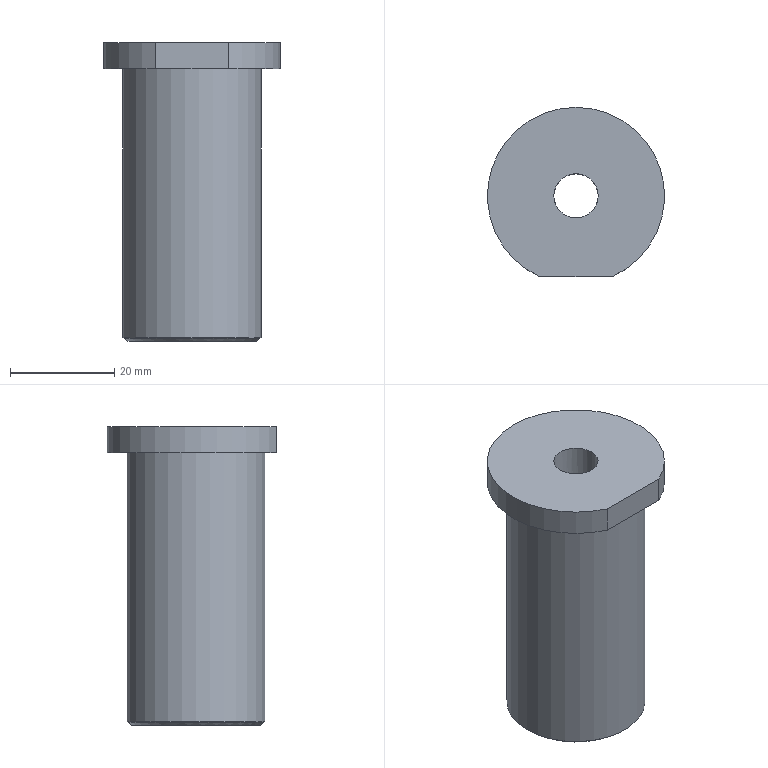Part | STEP file | SLIDE2-INSERT2_id610_x_t | 1 solid | 36 faces | box 34 x 32.5 x 57.321 mm | volume 25904 mm3 | plane 30 | cylinder 3 | other 2 | cone 1 | commonest cylinder face diameters 8.5 x1 26.5 x1 34 x1
STEP:
#1=CARTESIAN_POINT('',(18.501,-6.,56.682));
#2=VERTEX_POINT('',#1);
#3=CARTESIAN_POINT('',(18.617,-6.,56.682));
#4=VERTEX_POINT('',#3);
#5=CARTESIAN_POINT('',(22.656,-6.,56.682));
#6=DIRECTION('',(1.,0.,0.));
#7=VECTOR('',#6,1.);
#8=LINE('',#5,#7);
#9=EDGE_CURVE('',#2,#4,#8,.T.);
#10=ORIENTED_EDGE('',*,*,#9,.F.);
#11=CARTESIAN_POINT('',(18.501,-4.25,56.682));
#12=VERTEX_POINT('',#11);
#13=CARTESIAN_POINT('',(18.501,-6.,56.682));
#14=DIRECTION('',(0.,-1.,0.));
#15=VECTOR('',#14,1.);
#16=LINE('',#13,#15);
#17=EDGE_CURVE('',#12,#2,#16,.T.);
#18=ORIENTED_EDGE('',*,*,#17,.F.);
#19=CARTESIAN_POINT('',(18.617,-4.25,56.682));
#20=VERTEX_POINT('',#19);
#21=CARTESIAN_POINT('',(18.559,0.,56.682));
#22=DIRECTION('',(0.,0.,-1.));
#23=DIRECTION('',(1.,0.,0.));
#24=AXIS2_PLACEMENT_3D('',#21,#22,#23);
#25=CIRCLE('',#24,4.25);
#26=EDGE_CURVE('',#20,#12,#25,.T.);
#27=ORIENTED_EDGE('',*,*,#26,.F.);
#28=CARTESIAN_POINT('',(18.617,-6.,56.682));
#29=DIRECTION('',(0.,1.,0.));
#30=VECTOR('',#29,1.);
#31=LINE('',#28,#30);
#32=EDGE_CURVE('',#4,#20,#31,.T.);
#33=ORIENTED_EDGE('',*,*,#32,.F.);
#34=EDGE_LOOP('',(#10,#18,#27,#33));
#35=FACE_OUTER_BOUND('',#34,.T.);
#36=CARTESIAN_POINT('',(22.656,-6.,56.682));
#37=DIRECTION('',(0.,0.,1.));
#38=DIRECTION('',(1.,0.,0.));
#39=AXIS2_PLACEMENT_3D('',#36,#37,#38);
#40=PLANE('',#39);
#41=ADVANCED_FACE('',(#35),#40,.F.);
#42=CARTESIAN_POINT('',(18.501,6.,56.682));
#43=VERTEX_POINT('',#42);
#44=CARTESIAN_POINT('',(18.501,4.25,56.682));
#45=VERTEX_POINT('',#44);
#46=CARTESIAN_POINT('',(18.501,6.,56.682));
#47=DIRECTION('',(0.,-1.,0.));
#48=VECTOR('',#47,1.);
#49=LINE('',#46,#48);
#50=EDGE_CURVE('',#43,#45,#49,.T.);
#51=ORIENTED_EDGE('',*,*,#50,.F.);
#52=CARTESIAN_POINT('',(18.617,6.,56.682));
#53=VERTEX_POINT('',#52);
#54=CARTESIAN_POINT('',(22.656,6.,56.682));
#55=DIRECTION('',(-1.,0.,0.));
#56=VECTOR('',#55,1.);
#57=LINE('',#54,#56);
#58=EDGE_CURVE('',#53,#43,#57,.T.);
#59=ORIENTED_EDGE('',*,*,#58,.F.);
#60=CARTESIAN_POINT('',(18.617,4.25,56.682));
#61=VERTEX_POINT('',#60);
#62=CARTESIAN_POINT('',(18.617,6.,56.682));
#63=DIRECTION('',(0.,1.,0.));
#64=VECTOR('',#63,1.);
#65=LINE('',#62,#64);
#66=EDGE_CURVE('',#61,#53,#65,.T.);
#67=ORIENTED_EDGE('',*,*,#66,.F.);
#68=CARTESIAN_POINT('',(18.559,0.,56.682));
#69=DIRECTION('',(0.,0.,-1.));
#70=DIRECTION('',(1.,0.,0.));
#71=AXIS2_PLACEMENT_3D('',#68,#69,#70);
#72=CIRCLE('',#71,4.25);
#73=EDGE_CURVE('',#45,#61,#72,.T.);
#74=ORIENTED_EDGE('',*,*,#73,.F.);
#75=EDGE_LOOP('',(#51,#59,#67,#74));
#76=FACE_OUTER_BOUND('',#75,.T.);
#77=CARTESIAN_POINT('',(22.656,-6.,56.682));
#78=DIRECTION('',(0.,0.,1.));
#79=DIRECTION('',(1.,0.,0.));
#80=AXIS2_PLACEMENT_3D('',#77,#78,#79);
#81=PLANE('',#80);
#82=ADVANCED_FACE('',(#76),#81,.F.);
#83=CARTESIAN_POINT('',(25.977,-6.,18.682));
#84=VERTEX_POINT('',#83);
#85=CARTESIAN_POINT('',(25.977,-4.1,18.682));
#86=VERTEX_POINT('',#85);
#87=CARTESIAN_POINT('',(25.977,-6.,18.682));
#88=DIRECTION('',(0.,1.,0.));
#89=VECTOR('',#88,1.);
#90=LINE('',#87,#89);
#91=EDGE_CURVE('',#84,#86,#90,.T.);
#92=ORIENTED_EDGE('',*,*,#91,.F.);
#93=CARTESIAN_POINT('',(23.957,-6.,18.682));
#94=VERTEX_POINT('',#93);
#95=CARTESIAN_POINT('',(-30.,-6.,18.682));
#96=DIRECTION('',(-1.,0.,0.));
#97=VECTOR('',#96,1.);
#98=LINE('',#95,#97);
#99=EDGE_CURVE('',#84,#94,#98,.T.);
#100=ORIENTED_EDGE('',*,*,#99,.T.);
#101=CARTESIAN_POINT('',(23.957,-4.1,18.682));
#102=VERTEX_POINT('',#101);
#103=CARTESIAN_POINT('',(23.957,-6.,18.682));
#104=DIRECTION('',(0.,-1.,0.));
#105=VECTOR('',#104,1.);
#106=LINE('',#103,#105);
#107=EDGE_CURVE('',#102,#94,#106,.T.);
#108=ORIENTED_EDGE('',*,*,#107,.F.);
#109=CARTESIAN_POINT('',(-30.,-4.1,18.682));
#110=DIRECTION('',(-1.,0.,0.));
#111=VECTOR('',#110,1.);
#112=LINE('',#109,#111);
#113=EDGE_CURVE('',#86,#102,#112,.T.);
#114=ORIENTED_EDGE('',*,*,#113,.F.);
#115=EDGE_LOOP('',(#92,#100,#108,#114));
#116=FACE_OUTER_BOUND('',#115,.T.);
#117=CARTESIAN_POINT('',(25.977,-6.,18.682));
#118=DIRECTION('',(0.,0.,-1.));
#119=DIRECTION('',(-1.,0.,0.));
#120=AXIS2_PLACEMENT_3D('',#117,#118,#119);
#121=PLANE('',#120);
#122=ADVANCED_FACE('',(#116),#121,.T.);
#123=CARTESIAN_POINT('',(13.16,-6.,18.682));
#124=VERTEX_POINT('',#123);
#125=CARTESIAN_POINT('',(13.16,-4.1,18.682));
#126=VERTEX_POINT('',#125);
#127=CARTESIAN_POINT('',(13.16,-6.,18.682));
#128=DIRECTION('',(0.,1.,0.));
#129=VECTOR('',#128,1.);
#130=LINE('',#127,#129);
#131=EDGE_CURVE('',#124,#126,#130,.T.);
#132=ORIENTED_EDGE('',*,*,#131,.F.);
#133=CARTESIAN_POINT('',(11.14,-6.,18.682));
#134=VERTEX_POINT('',#133);
#135=CARTESIAN_POINT('',(-30.,-6.,18.682));
#136=DIRECTION('',(-1.,0.,0.));
#137=VECTOR('',#136,1.);
#138=LINE('',#135,#137);
#139=EDGE_CURVE('',#124,#134,#138,.T.);
#140=ORIENTED_EDGE('',*,*,#139,.T.);
#141=CARTESIAN_POINT('',(11.14,-4.1,18.682));
#142=VERTEX_POINT('',#141);
#143=CARTESIAN_POINT('',(11.14,-6.,18.682));
#144=DIRECTION('',(0.,-1.,0.));
#145=VECTOR('',#144,1.);
#146=LINE('',#143,#145);
#147=EDGE_CURVE('',#142,#134,#146,.T.);
#148=ORIENTED_EDGE('',*,*,#147,.F.);
#149=CARTESIAN_POINT('',(-30.,-4.1,18.682));
#150=DIRECTION('',(-1.,0.,0.));
#151=VECTOR('',#150,1.);
#152=LINE('',#149,#151);
#153=EDGE_CURVE('',#126,#142,#152,.T.);
#154=ORIENTED_EDGE('',*,*,#153,.F.);
#155=EDGE_LOOP('',(#132,#140,#148,#154));
#156=FACE_OUTER_BOUND('',#155,.T.);
#157=CARTESIAN_POINT('',(13.16,-6.,18.682));
#158=DIRECTION('',(0.,0.,-1.));
#159=DIRECTION('',(-1.,0.,0.));
#160=AXIS2_PLACEMENT_3D('',#157,#158,#159);
#161=PLANE('',#160);
#162=ADVANCED_FACE('',(#156),#161,.T.);
#163=ORIENTED_EDGE('',*,*,#147,.T.);
#164=CARTESIAN_POINT('',(16.481,-6.,56.682));
#165=VERTEX_POINT('',#164);
#166=CARTESIAN_POINT('',(11.14,-6.,18.682));
#167=DIRECTION('',(0.1392,0.,0.9903));
#168=VECTOR('',#167,1.);
#169=LINE('',#166,#168);
#170=EDGE_CURVE('',#134,#165,#169,.T.);
#171=ORIENTED_EDGE('',*,*,#170,.T.);
#172=CARTESIAN_POINT('',(16.481,-4.1,56.682));
#173=VERTEX_POINT('',#172);
#174=CARTESIAN_POINT('',(16.481,-6.,56.682));
#175=DIRECTION('',(0.,1.,0.));
#176=VECTOR('',#175,1.);
#177=LINE('',#174,#176);
#178=EDGE_CURVE('',#165,#173,#177,.T.);
#179=ORIENTED_EDGE('',*,*,#178,.T.);
#180=CARTESIAN_POINT('',(11.14,-4.1,18.682));
#181=DIRECTION('',(0.1392,0.,0.9903));
#182=VECTOR('',#181,1.);
#183=LINE('',#180,#182);
#184=EDGE_CURVE('',#142,#173,#183,.T.);
#185=ORIENTED_EDGE('',*,*,#184,.F.);
#186=EDGE_LOOP('',(#163,#171,#179,#185));
#187=FACE_OUTER_BOUND('',#186,.T.);
#188=CARTESIAN_POINT('',(11.14,-6.,18.682));
#189=DIRECTION('',(-0.9903,0.,0.1392));
#190=DIRECTION('',(0.1392,0.,0.9903));
#191=AXIS2_PLACEMENT_3D('',#188,#189,#190);
#192=PLANE('',#191);
#193=ADVANCED_FACE('',(#187),#192,.T.);
#194=CARTESIAN_POINT('',(20.636,-4.1,56.682));
#195=VERTEX_POINT('',#194);
#196=CARTESIAN_POINT('',(20.636,-6.,56.682));
#197=VERTEX_POINT('',#196);
#198=CARTESIAN_POINT('',(20.636,-6.,56.682));
#199=DIRECTION('',(0.,-1.,0.));
#200=VECTOR('',#199,1.);
#201=LINE('',#198,#200);
#202=EDGE_CURVE('',#195,#197,#201,.T.);
#203=ORIENTED_EDGE('',*,*,#202,.T.);
#204=CARTESIAN_POINT('',(20.636,-6.,56.682));
#205=DIRECTION('',(0.1392,0.,-0.9903));
#206=VECTOR('',#205,1.);
#207=LINE('',#204,#206);
#208=EDGE_CURVE('',#197,#84,#207,.T.);
#209=ORIENTED_EDGE('',*,*,#208,.T.);
#210=ORIENTED_EDGE('',*,*,#91,.T.);
#211=CARTESIAN_POINT('',(20.636,-4.1,56.682));
#212=DIRECTION('',(0.1392,0.,-0.9903));
#213=VECTOR('',#212,1.);
#214=LINE('',#211,#213);
#215=EDGE_CURVE('',#195,#86,#214,.T.);
#216=ORIENTED_EDGE('',*,*,#215,.F.);
#217=EDGE_LOOP('',(#203,#209,#210,#216));
#218=FACE_OUTER_BOUND('',#217,.T.);
#219=CARTESIAN_POINT('',(20.636,-6.,56.682));
#220=DIRECTION('',(0.9903,0.,0.1392));
#221=DIRECTION('',(0.1392,0.,-0.9903));
#222=AXIS2_PLACEMENT_3D('',#219,#220,#221);
#223=PLANE('',#222);
#224=ADVANCED_FACE('',(#218),#223,.T.);
#225=CARTESIAN_POINT('',(11.14,6.,18.682));
#226=VERTEX_POINT('',#225);
#227=CARTESIAN_POINT('',(11.14,4.1,18.682));
#228=VERTEX_POINT('',#227);
#229=CARTESIAN_POINT('',(11.14,6.,18.682));
#230=DIRECTION('',(0.,-1.,0.));
#231=VECTOR('',#230,1.);
#232=LINE('',#229,#231);
#233=EDGE_CURVE('',#226,#228,#232,.T.);
#234=ORIENTED_EDGE('',*,*,#233,.F.);
#235=CARTESIAN_POINT('',(13.16,6.,18.682));
#236=VERTEX_POINT('',#235);
#237=CARTESIAN_POINT('',(-30.,6.,18.682));
#238=DIRECTION('',(-1.,0.,0.));
#239=VECTOR('',#238,1.);
#240=LINE('',#237,#239);
#241=EDGE_CURVE('',#236,#226,#240,.T.);
#242=ORIENTED_EDGE('',*,*,#241,.F.);
#243=CARTESIAN_POINT('',(13.16,4.1,18.682));
#244=VERTEX_POINT('',#243);
#245=CARTESIAN_POINT('',(13.16,6.,18.682));
#246=DIRECTION('',(0.,1.,0.));
#247=VECTOR('',#246,1.);
#248=LINE('',#245,#247);
#249=EDGE_CURVE('',#244,#236,#248,.T.);
#250=ORIENTED_EDGE('',*,*,#249,.F.);
#251=CARTESIAN_POINT('',(-30.,4.1,18.682));
#252=DIRECTION('',(1.,0.,0.));
#253=VECTOR('',#252,1.);
#254=LINE('',#251,#253);
#255=EDGE_CURVE('',#228,#244,#254,.T.);
#256=ORIENTED_EDGE('',*,*,#255,.F.);
#257=EDGE_LOOP('',(#234,#242,#250,#256));
#258=FACE_OUTER_BOUND('',#257,.T.);
#259=CARTESIAN_POINT('',(11.14,6.,18.682));
#260=DIRECTION('',(0.,0.,-1.));
#261=DIRECTION('',(-1.,0.,0.));
#262=AXIS2_PLACEMENT_3D('',#259,#260,#261);
#263=PLANE('',#262);
#264=ADVANCED_FACE('',(#258),#263,.T.);
#265=CARTESIAN_POINT('',(16.481,4.1,56.682));
#266=VERTEX_POINT('',#265);
#267=CARTESIAN_POINT('',(16.481,6.,56.682));
#268=VERTEX_POINT('',#267);
#269=CARTESIAN_POINT('',(16.481,-6.,56.682));
#270=DIRECTION('',(0.,1.,0.));
#271=VECTOR('',#270,1.);
#272=LINE('',#269,#271);
#273=EDGE_CURVE('',#266,#268,#272,.T.);
#274=ORIENTED_EDGE('',*,*,#273,.T.);
#275=CARTESIAN_POINT('',(11.14,6.,18.682));
#276=DIRECTION('',(0.1392,0.,0.9903));
#277=VECTOR('',#276,1.);
#278=LINE('',#275,#277);
#279=EDGE_CURVE('',#226,#268,#278,.T.);
#280=ORIENTED_EDGE('',*,*,#279,.F.);
#281=ORIENTED_EDGE('',*,*,#233,.T.);
#282=CARTESIAN_POINT('',(16.481,4.1,56.682));
#283=DIRECTION('',(-0.1392,0.,-0.9903));
#284=VECTOR('',#283,1.);
#285=LINE('',#282,#284);
#286=EDGE_CURVE('',#266,#228,#285,.T.);
#287=ORIENTED_EDGE('',*,*,#286,.F.);
#288=EDGE_LOOP('',(#274,#280,#281,#287));
#289=FACE_OUTER_BOUND('',#288,.T.);
#290=CARTESIAN_POINT('',(16.481,6.,56.682));
#291=DIRECTION('',(-0.9903,0.,0.1392));
#292=DIRECTION('',(0.1392,0.,0.9903));
#293=AXIS2_PLACEMENT_3D('',#290,#291,#292);
#294=PLANE('',#293);
#295=ADVANCED_FACE('',(#289),#294,.T.);
#296=CARTESIAN_POINT('',(25.977,6.,18.682));
#297=VERTEX_POINT('',#296);
#298=CARTESIAN_POINT('',(25.977,4.1,18.682));
#299=VERTEX_POINT('',#298);
#300=CARTESIAN_POINT('',(25.977,6.,18.682));
#301=DIRECTION('',(0.,-1.,0.));
#302=VECTOR('',#301,1.);
#303=LINE('',#300,#302);
#304=EDGE_CURVE('',#297,#299,#303,.T.);
#305=ORIENTED_EDGE('',*,*,#304,.F.);
#306=CARTESIAN_POINT('',(20.636,6.,56.682));
#307=VERTEX_POINT('',#306);
#308=CARTESIAN_POINT('',(20.636,6.,56.682));
#309=DIRECTION('',(0.1392,0.,-0.9903));
#310=VECTOR('',#309,1.);
#311=LINE('',#308,#310);
#312=EDGE_CURVE('',#307,#297,#311,.T.);
#313=ORIENTED_EDGE('',*,*,#312,.F.);
#314=CARTESIAN_POINT('',(20.636,4.1,56.682));
#315=VERTEX_POINT('',#314);
#316=CARTESIAN_POINT('',(20.636,-6.,56.682));
#317=DIRECTION('',(0.,-1.,0.));
#318=VECTOR('',#317,1.);
#319=LINE('',#316,#318);
#320=EDGE_CURVE('',#307,#315,#319,.T.);
#321=ORIENTED_EDGE('',*,*,#320,.T.);
#322=CARTESIAN_POINT('',(25.977,4.1,18.682));
#323=DIRECTION('',(-0.1392,0.,0.9903));
#324=VECTOR('',#323,1.);
#325=LINE('',#322,#324);
#326=EDGE_CURVE('',#299,#315,#325,.T.);
#327=ORIENTED_EDGE('',*,*,#326,.F.);
#328=EDGE_LOOP('',(#305,#313,#321,#327));
#329=FACE_OUTER_BOUND('',#328,.T.);
#330=CARTESIAN_POINT('',(25.977,6.,18.682));
#331=DIRECTION('',(0.9903,0.,0.1392));
#332=DIRECTION('',(0.1392,0.,-0.9903));
#333=AXIS2_PLACEMENT_3D('',#330,#331,#332);
#334=PLANE('',#333);
#335=ADVANCED_FACE('',(#329),#334,.T.);
#336=CARTESIAN_POINT('',(23.957,6.,18.682));
#337=VERTEX_POINT('',#336);
#338=CARTESIAN_POINT('',(23.957,4.1,18.682));
#339=VERTEX_POINT('',#338);
#340=CARTESIAN_POINT('',(23.957,6.,18.682));
#341=DIRECTION('',(0.,-1.,0.));
#342=VECTOR('',#341,1.);
#343=LINE('',#340,#342);
#344=EDGE_CURVE('',#337,#339,#343,.T.);
#345=ORIENTED_EDGE('',*,*,#344,.F.);
#346=CARTESIAN_POINT('',(-30.,6.,18.682));
#347=DIRECTION('',(-1.,0.,0.));
#348=VECTOR('',#347,1.);
#349=LINE('',#346,#348);
#350=EDGE_CURVE('',#297,#337,#349,.T.);
#351=ORIENTED_EDGE('',*,*,#350,.F.);
#352=ORIENTED_EDGE('',*,*,#304,.T.);
#353=CARTESIAN_POINT('',(-30.,4.1,18.682));
#354=DIRECTION('',(1.,0.,0.));
#355=VECTOR('',#354,1.);
#356=LINE('',#353,#355);
#357=EDGE_CURVE('',#339,#299,#356,.T.);
#358=ORIENTED_EDGE('',*,*,#357,.F.);
#359=EDGE_LOOP('',(#345,#351,#352,#358));
#360=FACE_OUTER_BOUND('',#359,.T.);
#361=CARTESIAN_POINT('',(23.957,6.,18.682));
#362=DIRECTION('',(0.,0.,-1.));
#363=DIRECTION('',(-1.,0.,0.));
#364=AXIS2_PLACEMENT_3D('',#361,#362,#363);
#365=PLANE('',#364);
#366=ADVANCED_FACE('',(#360),#365,.T.);
#367=ORIENTED_EDGE('',*,*,#50,.T.);
#368=CARTESIAN_POINT('',(17.439,4.1,49.132));
#369=VERTEX_POINT('',#368);
#370=CARTESIAN_POINT('',(18.559,0.,57.095));
#371=DIRECTION('',(-0.9903,0.,0.1392));
#372=DIRECTION('',(0.1392,0.,0.9903));
#373=AXIS2_PLACEMENT_3D('',#370,#371,#372);
#374=ELLIPSE('',#373,30.538,4.25);
#375=EDGE_CURVE('',#45,#369,#374,.T.);
#376=ORIENTED_EDGE('',*,*,#375,.T.);
#377=CARTESIAN_POINT('',(13.16,4.1,18.682));
#378=DIRECTION('',(0.1392,0.,0.9903));
#379=VECTOR('',#378,1.);
#380=LINE('',#377,#379);
#381=EDGE_CURVE('',#244,#369,#380,.T.);
#382=ORIENTED_EDGE('',*,*,#381,.F.);
#383=ORIENTED_EDGE('',*,*,#249,.T.);
#384=CARTESIAN_POINT('',(18.501,6.,56.682));
#385=DIRECTION('',(-0.1392,0.,-0.9903));
#386=VECTOR('',#385,1.);
#387=LINE('',#384,#386);
#388=EDGE_CURVE('',#43,#236,#387,.T.);
#389=ORIENTED_EDGE('',*,*,#388,.F.);
#390=EDGE_LOOP('',(#367,#376,#382,#383,#389));
#391=FACE_OUTER_BOUND('',#390,.T.);
#392=CARTESIAN_POINT('',(13.16,6.,18.682));
#393=DIRECTION('',(0.9903,0.,-0.1392));
#394=DIRECTION('',(-0.1392,0.,-0.9903));
#395=AXIS2_PLACEMENT_3D('',#392,#393,#394);
#396=PLANE('',#395);
#397=ADVANCED_FACE('',(#391),#396,.T.);
#398=ORIENTED_EDGE('',*,*,#381,.T.);
#399=CARTESIAN_POINT('',(17.439,4.1,56.682));
#400=VERTEX_POINT('',#399);
#401=CARTESIAN_POINT('',(17.439,4.1,62.003));
#402=DIRECTION('',(0.,0.,1.));
#403=VECTOR('',#402,1.);
#404=LINE('',#401,#403);
#405=EDGE_CURVE('',#369,#400,#404,.T.);
#406=ORIENTED_EDGE('',*,*,#405,.T.);
#407=CARTESIAN_POINT('',(22.656,4.1,56.682));
#408=DIRECTION('',(-1.,0.,0.));
#409=VECTOR('',#408,1.);
#410=LINE('',#407,#409);
#411=EDGE_CURVE('',#400,#266,#410,.T.);
#412=ORIENTED_EDGE('',*,*,#411,.T.);
#413=ORIENTED_EDGE('',*,*,#286,.T.);
#414=ORIENTED_EDGE('',*,*,#255,.T.);
#415=EDGE_LOOP('',(#398,#406,#412,#413,#414));
#416=FACE_OUTER_BOUND('',#415,.T.);
#417=CARTESIAN_POINT('',(-30.,4.1,14.682));
#418=DIRECTION('',(0.,-1.,0.));
#419=DIRECTION('',(0.,0.,-1.));
#420=AXIS2_PLACEMENT_3D('',#417,#418,#419);
#421=PLANE('',#420);
#422=ADVANCED_FACE('',(#416),#421,.T.);
#423=CARTESIAN_POINT('',(14.461,6.,56.682));
#424=VERTEX_POINT('',#423);
#425=CARTESIAN_POINT('',(-30.,6.,56.682));
#426=DIRECTION('',(-1.,0.,0.));
#427=VECTOR('',#426,1.);
#428=LINE('',#425,#427);
#429=EDGE_CURVE('',#268,#424,#428,.T.);
#430=ORIENTED_EDGE('',*,*,#429,.F.);
#431=ORIENTED_EDGE('',*,*,#273,.F.);
#432=ORIENTED_EDGE('',*,*,#411,.F.);
#433=CARTESIAN_POINT('',(14.461,1.129,56.682));
#434=VERTEX_POINT('',#433);
#435=CARTESIAN_POINT('',(18.559,0.,56.682));
#436=DIRECTION('',(0.,0.,1.));
#437=DIRECTION('',(1.,0.,0.));
#438=AXIS2_PLACEMENT_3D('',#435,#436,#437);
#439=CIRCLE('',#438,4.25);
#440=EDGE_CURVE('',#400,#434,#439,.T.);
#441=ORIENTED_EDGE('',*,*,#440,.T.);
#442=CARTESIAN_POINT('',(14.461,-6.,56.682));
#443=DIRECTION('',(0.,1.,0.));
#444=VECTOR('',#443,1.);
#445=LINE('',#442,#444);
#446=EDGE_CURVE('',#434,#424,#445,.T.);
#447=ORIENTED_EDGE('',*,*,#446,.T.);
#448=EDGE_LOOP('',(#430,#431,#432,#441,#447));
#449=FACE_OUTER_BOUND('',#448,.T.);
#450=CARTESIAN_POINT('',(22.656,-6.,56.682));
#451=DIRECTION('',(0.,0.,1.));
#452=DIRECTION('',(1.,0.,0.));
#453=AXIS2_PLACEMENT_3D('',#450,#451,#452);
#454=PLANE('',#453);
#455=ADVANCED_FACE('',(#449),#454,.F.);
#456=ORIENTED_EDGE('',*,*,#178,.F.);
#457=CARTESIAN_POINT('',(14.461,-6.,56.682));
#458=VERTEX_POINT('',#457);
#459=CARTESIAN_POINT('',(-30.,-6.,56.682));
#460=DIRECTION('',(-1.,0.,0.));
#461=VECTOR('',#460,1.);
#462=LINE('',#459,#461);
#463=EDGE_CURVE('',#165,#458,#462,.T.);
#464=ORIENTED_EDGE('',*,*,#463,.T.);
#465=CARTESIAN_POINT('',(14.461,-1.129,56.682));
#466=VERTEX_POINT('',#465);
#467=CARTESIAN_POINT('',(14.461,-6.,56.682));
#468=DIRECTION('',(0.,1.,0.));
#469=VECTOR('',#468,1.);
#470=LINE('',#467,#469);
#471=EDGE_CURVE('',#458,#466,#470,.T.);
#472=ORIENTED_EDGE('',*,*,#471,.T.);
#473=CARTESIAN_POINT('',(17.439,-4.1,56.682));
#474=VERTEX_POINT('',#473);
#475=CARTESIAN_POINT('',(18.559,0.,56.682));
#476=DIRECTION('',(0.,0.,1.));
#477=DIRECTION('',(1.,0.,0.));
#478=AXIS2_PLACEMENT_3D('',#475,#476,#477);
#479=CIRCLE('',#478,4.25);
#480=EDGE_CURVE('',#466,#474,#479,.T.);
#481=ORIENTED_EDGE('',*,*,#480,.T.);
#482=CARTESIAN_POINT('',(-30.,-4.1,56.682));
#483=DIRECTION('',(1.,0.,0.));
#484=VECTOR('',#483,1.);
#485=LINE('',#482,#484);
#486=EDGE_CURVE('',#173,#474,#485,.T.);
#487=ORIENTED_EDGE('',*,*,#486,.F.);
#488=EDGE_LOOP('',(#456,#464,#472,#481,#487));
#489=FACE_OUTER_BOUND('',#488,.T.);
#490=CARTESIAN_POINT('',(22.656,-6.,56.682));
#491=DIRECTION('',(0.,0.,1.));
#492=DIRECTION('',(1.,0.,0.));
#493=AXIS2_PLACEMENT_3D('',#490,#491,#492);
#494=PLANE('',#493);
#495=ADVANCED_FACE('',(#489),#494,.F.);
#496=ORIENTED_EDGE('',*,*,#486,.T.);
#497=CARTESIAN_POINT('',(17.439,-4.1,49.132));
#498=VERTEX_POINT('',#497);
#499=CARTESIAN_POINT('',(17.439,-4.1,62.003));
#500=DIRECTION('',(0.,0.,-1.));
#501=VECTOR('',#500,1.);
#502=LINE('',#499,#501);
#503=EDGE_CURVE('',#474,#498,#502,.T.);
#504=ORIENTED_EDGE('',*,*,#503,.T.);
#505=CARTESIAN_POINT('',(18.501,-4.1,56.682));
#506=DIRECTION('',(0.1392,0.,0.9903));
#507=VECTOR('',#506,1.);
#508=LINE('',#505,#507);
#509=EDGE_CURVE('',#126,#498,#508,.T.);
#510=ORIENTED_EDGE('',*,*,#509,.F.);
#511=ORIENTED_EDGE('',*,*,#153,.T.);
#512=ORIENTED_EDGE('',*,*,#184,.T.);
#513=EDGE_LOOP('',(#496,#504,#510,#511,#512));
#514=FACE_OUTER_BOUND('',#513,.T.);
#515=CARTESIAN_POINT('',(-30.,-4.1,14.682));
#516=DIRECTION('',(0.,1.,0.));
#517=DIRECTION('',(0.,0.,1.));
#518=AXIS2_PLACEMENT_3D('',#515,#516,#517);
#519=PLANE('',#518);
#520=ADVANCED_FACE('',(#514),#519,.T.);
#521=ORIENTED_EDGE('',*,*,#509,.T.);
#522=CARTESIAN_POINT('',(18.559,0.,57.095));
#523=DIRECTION('',(-0.9903,0.,0.1392));
#524=DIRECTION('',(0.1392,0.,0.9903));
#525=AXIS2_PLACEMENT_3D('',#522,#523,#524);
#526=ELLIPSE('',#525,30.538,4.25);
#527=EDGE_CURVE('',#498,#12,#526,.T.);
#528=ORIENTED_EDGE('',*,*,#527,.T.);
#529=ORIENTED_EDGE('',*,*,#17,.T.);
#530=CARTESIAN_POINT('',(18.501,-6.,56.682));
#531=DIRECTION('',(-0.1392,0.,-0.9903));
#532=VECTOR('',#531,1.);
#533=LINE('',#530,#532);
#534=EDGE_CURVE('',#2,#124,#533,.T.);
#535=ORIENTED_EDGE('',*,*,#534,.T.);
#536=ORIENTED_EDGE('',*,*,#131,.T.);
#537=EDGE_LOOP('',(#521,#528,#529,#535,#536));
#538=FACE_OUTER_BOUND('',#537,.T.);
#539=CARTESIAN_POINT('',(18.501,-6.,56.682));
#540=DIRECTION('',(0.9903,0.,-0.1392));
#541=DIRECTION('',(-0.1392,0.,-0.9903));
#542=AXIS2_PLACEMENT_3D('',#539,#540,#541);
#543=PLANE('',#542);
#544=ADVANCED_FACE('',(#538),#543,.T.);
#545=ORIENTED_EDGE('',*,*,#32,.T.);
#546=CARTESIAN_POINT('',(19.678,-4.1,49.132));
#547=VERTEX_POINT('',#546);
#548=CARTESIAN_POINT('',(18.559,0.,57.095));
#549=DIRECTION('',(0.9903,0.,0.1392));
#550=DIRECTION('',(-0.1392,0.,0.9903));
#551=AXIS2_PLACEMENT_3D('',#548,#549,#550);
#552=ELLIPSE('',#551,30.538,4.25);
#553=EDGE_CURVE('',#20,#547,#552,.T.);
#554=ORIENTED_EDGE('',*,*,#553,.T.);
#555=CARTESIAN_POINT('',(23.957,-4.1,18.682));
#556=DIRECTION('',(-0.1392,0.,0.9903));
#557=VECTOR('',#556,1.);
#558=LINE('',#555,#557);
#559=EDGE_CURVE('',#102,#547,#558,.T.);
#560=ORIENTED_EDGE('',*,*,#559,.F.);
#561=ORIENTED_EDGE('',*,*,#107,.T.);
#562=CARTESIAN_POINT('',(23.957,-6.,18.682));
#563=DIRECTION('',(-0.1392,0.,0.9903));
#564=VECTOR('',#563,1.);
#565=LINE('',#562,#564);
#566=EDGE_CURVE('',#94,#4,#565,.T.);
#567=ORIENTED_EDGE('',*,*,#566,.T.);
#568=EDGE_LOOP('',(#545,#554,#560,#561,#567));
#569=FACE_OUTER_BOUND('',#568,.T.);
#570=CARTESIAN_POINT('',(23.957,-6.,18.682));
#571=DIRECTION('',(-0.9903,0.,-0.1392));
#572=DIRECTION('',(-0.1392,0.,0.9903));
#573=AXIS2_PLACEMENT_3D('',#570,#571,#572);
#574=PLANE('',#573);
#575=ADVANCED_FACE('',(#569),#574,.T.);
#576=ORIENTED_EDGE('',*,*,#559,.T.);
#577=CARTESIAN_POINT('',(19.678,-4.1,56.682));
#578=VERTEX_POINT('',#577);
#579=CARTESIAN_POINT('',(19.678,-4.1,62.003));
#580=DIRECTION('',(0.,0.,1.));
#581=VECTOR('',#580,1.);
#582=LINE('',#579,#581);
#583=EDGE_CURVE('',#547,#578,#582,.T.);
#584=ORIENTED_EDGE('',*,*,#583,.T.);
#585=CARTESIAN_POINT('',(22.656,-4.1,56.682));
#586=DIRECTION('',(1.,0.,0.));
#587=VECTOR('',#586,1.);
#588=LINE('',#585,#587);
#589=EDGE_CURVE('',#578,#195,#588,.T.);
#590=ORIENTED_EDGE('',*,*,#589,.T.);
#591=ORIENTED_EDGE('',*,*,#215,.T.);
#592=ORIENTED_EDGE('',*,*,#113,.T.);
#593=EDGE_LOOP('',(#576,#584,#590,#591,#592));
#594=FACE_OUTER_BOUND('',#593,.T.);
#595=CARTESIAN_POINT('',(-30.,-4.1,14.682));
#596=DIRECTION('',(0.,1.,0.));
#597=DIRECTION('',(0.,0.,1.));
#598=AXIS2_PLACEMENT_3D('',#595,#596,#597);
#599=PLANE('',#598);
#600=ADVANCED_FACE('',(#594),#599,.T.);
#601=CARTESIAN_POINT('',(22.656,-6.,56.682));
#602=VERTEX_POINT('',#601);
#603=CARTESIAN_POINT('',(-30.,-6.,56.682));
#604=DIRECTION('',(-1.,0.,0.));
#605=VECTOR('',#604,1.);
#606=LINE('',#603,#605);
#607=EDGE_CURVE('',#602,#197,#606,.T.);
#608=ORIENTED_EDGE('',*,*,#607,.T.);
#609=ORIENTED_EDGE('',*,*,#202,.F.);
#610=ORIENTED_EDGE('',*,*,#589,.F.);
#611=CARTESIAN_POINT('',(22.656,-1.129,56.682));
#612=VERTEX_POINT('',#611);
#613=CARTESIAN_POINT('',(18.559,0.,56.682));
#614=DIRECTION('',(0.,0.,1.));
#615=DIRECTION('',(1.,0.,0.));
#616=AXIS2_PLACEMENT_3D('',#613,#614,#615);
#617=CIRCLE('',#616,4.25);
#618=EDGE_CURVE('',#578,#612,#617,.T.);
#619=ORIENTED_EDGE('',*,*,#618,.T.);
#620=CARTESIAN_POINT('',(22.656,-6.,56.682));
#621=DIRECTION('',(0.,-1.,0.));
#622=VECTOR('',#621,1.);
#623=LINE('',#620,#622);
#624=EDGE_CURVE('',#612,#602,#623,.T.);
#625=ORIENTED_EDGE('',*,*,#624,.T.);
#626=EDGE_LOOP('',(#608,#609,#610,#619,#625));
#627=FACE_OUTER_BOUND('',#626,.T.);
#628=CARTESIAN_POINT('',(22.656,-6.,56.682));
#629=DIRECTION('',(0.,0.,1.));
#630=DIRECTION('',(1.,0.,0.));
#631=AXIS2_PLACEMENT_3D('',#628,#629,#630);
#632=PLANE('',#631);
#633=ADVANCED_FACE('',(#627),#632,.F.);
#634=ORIENTED_EDGE('',*,*,#320,.F.);
#635=CARTESIAN_POINT('',(22.656,6.,56.682));
#636=VERTEX_POINT('',#635);
#637=CARTESIAN_POINT('',(-30.,6.,56.682));
#638=DIRECTION('',(-1.,0.,0.));
#639=VECTOR('',#638,1.);
#640=LINE('',#637,#639);
#641=EDGE_CURVE('',#636,#307,#640,.T.);
#642=ORIENTED_EDGE('',*,*,#641,.F.);
#643=CARTESIAN_POINT('',(22.656,1.129,56.682));
#644=VERTEX_POINT('',#643);
#645=CARTESIAN_POINT('',(22.656,-6.,56.682));
#646=DIRECTION('',(0.,-1.,0.));
#647=VECTOR('',#646,1.);
#648=LINE('',#645,#647);
#649=EDGE_CURVE('',#636,#644,#648,.T.);
#650=ORIENTED_EDGE('',*,*,#649,.T.);
#651=CARTESIAN_POINT('',(19.678,4.1,56.682));
#652=VERTEX_POINT('',#651);
#653=CARTESIAN_POINT('',(18.559,0.,56.682));
#654=DIRECTION('',(0.,0.,1.));
#655=DIRECTION('',(1.,0.,0.));
#656=AXIS2_PLACEMENT_3D('',#653,#654,#655);
#657=CIRCLE('',#656,4.25);
#658=EDGE_CURVE('',#644,#652,#657,.T.);
#659=ORIENTED_EDGE('',*,*,#658,.T.);
#660=CARTESIAN_POINT('',(-30.,4.1,56.682));
#661=DIRECTION('',(-1.,0.,0.));
#662=VECTOR('',#661,1.);
#663=LINE('',#660,#662);
#664=EDGE_CURVE('',#315,#652,#663,.T.);
#665=ORIENTED_EDGE('',*,*,#664,.F.);
#666=EDGE_LOOP('',(#634,#642,#650,#659,#665));
#667=FACE_OUTER_BOUND('',#666,.T.);
#668=CARTESIAN_POINT('',(22.656,-6.,56.682));
#669=DIRECTION('',(0.,0.,1.));
#670=DIRECTION('',(1.,0.,0.));
#671=AXIS2_PLACEMENT_3D('',#668,#669,#670);
#672=PLANE('',#671);
#673=ADVANCED_FACE('',(#667),#672,.F.);
#674=ORIENTED_EDGE('',*,*,#664,.T.);
#675=CARTESIAN_POINT('',(19.678,4.1,49.132));
#676=VERTEX_POINT('',#675);
#677=CARTESIAN_POINT('',(19.678,4.1,62.003));
#678=DIRECTION('',(0.,0.,-1.));
#679=VECTOR('',#678,1.);
#680=LINE('',#677,#679);
#681=EDGE_CURVE('',#652,#676,#680,.T.);
#682=ORIENTED_EDGE('',*,*,#681,.T.);
#683=CARTESIAN_POINT('',(18.617,4.1,56.682));
#684=DIRECTION('',(-0.1392,0.,0.9903));
#685=VECTOR('',#684,1.);
#686=LINE('',#683,#685);
#687=EDGE_CURVE('',#339,#676,#686,.T.);
#688=ORIENTED_EDGE('',*,*,#687,.F.);
#689=ORIENTED_EDGE('',*,*,#357,.T.);
#690=ORIENTED_EDGE('',*,*,#326,.T.);
#691=EDGE_LOOP('',(#674,#682,#688,#689,#690));
#692=FACE_OUTER_BOUND('',#691,.T.);
#693=CARTESIAN_POINT('',(-30.,4.1,14.682));
#694=DIRECTION('',(0.,-1.,0.));
#695=DIRECTION('',(0.,0.,-1.));
#696=AXIS2_PLACEMENT_3D('',#693,#694,#695);
#697=PLANE('',#696);
#698=ADVANCED_FACE('',(#692),#697,.T.);
#699=ORIENTED_EDGE('',*,*,#687,.T.);
#700=CARTESIAN_POINT('',(18.559,0.,57.095));
#701=DIRECTION('',(0.9903,0.,0.1392));
#702=DIRECTION('',(-0.1392,0.,0.9903));
#703=AXIS2_PLACEMENT_3D('',#700,#701,#702);
#704=ELLIPSE('',#703,30.538,4.25);
#705=EDGE_CURVE('',#676,#61,#704,.T.);
#706=ORIENTED_EDGE('',*,*,#705,.T.);
#707=ORIENTED_EDGE('',*,*,#66,.T.);
#708=CARTESIAN_POINT('',(23.957,6.,18.682));
#709=DIRECTION('',(-0.1392,0.,0.9903));
#710=VECTOR('',#709,1.);
#711=LINE('',#708,#710);
#712=EDGE_CURVE('',#337,#53,#711,.T.);
#713=ORIENTED_EDGE('',*,*,#712,.F.);
#714=ORIENTED_EDGE('',*,*,#344,.T.);
#715=EDGE_LOOP('',(#699,#706,#707,#713,#714));
#716=FACE_OUTER_BOUND('',#715,.T.);
#717=CARTESIAN_POINT('',(18.617,6.,56.682));
#718=DIRECTION('',(-0.9903,0.,-0.1392));
#719=DIRECTION('',(-0.1392,0.,0.9903));
#720=AXIS2_PLACEMENT_3D('',#717,#718,#719);
#721=PLANE('',#720);
#722=ADVANCED_FACE('',(#716),#721,.T.);
#723=ORIENTED_EDGE('',*,*,#607,.F.);
#724=CARTESIAN_POINT('',(28.559,-6.,14.682));
#725=VERTEX_POINT('',#724);
#726=CARTESIAN_POINT('',(29.318,-6.,9.28));
#727=DIRECTION('',(0.1392,0.,-0.9903));
#728=VECTOR('',#727,1.);
#729=LINE('',#726,#728);
#730=EDGE_CURVE('',#602,#725,#729,.T.);
#731=ORIENTED_EDGE('',*,*,#730,.T.);
#732=CARTESIAN_POINT('',(8.559,-6.,14.682));
#733=VERTEX_POINT('',#732);
#734=CARTESIAN_POINT('',(-30.,-6.,14.682));
#735=DIRECTION('',(-1.,0.,0.));
#736=VECTOR('',#735,1.);
#737=LINE('',#734,#736);
#738=EDGE_CURVE('',#725,#733,#737,.T.);
#739=ORIENTED_EDGE('',*,*,#738,.T.);
#740=CARTESIAN_POINT('',(14.461,-6.,56.682));
#741=DIRECTION('',(0.1392,0.,0.9903));
#742=VECTOR('',#741,1.);
#743=LINE('',#740,#742);
#744=EDGE_CURVE('',#733,#458,#743,.T.);
#745=ORIENTED_EDGE('',*,*,#744,.T.);
#746=ORIENTED_EDGE('',*,*,#463,.F.);
#747=ORIENTED_EDGE('',*,*,#170,.F.);
#748=ORIENTED_EDGE('',*,*,#139,.F.);
#749=ORIENTED_EDGE('',*,*,#534,.F.);
#750=ORIENTED_EDGE('',*,*,#9,.T.);
#751=ORIENTED_EDGE('',*,*,#566,.F.);
#752=ORIENTED_EDGE('',*,*,#99,.F.);
#753=ORIENTED_EDGE('',*,*,#208,.F.);
#754=EDGE_LOOP('',(#723,#731,#739,#745,#746,#747,#748,#749,#750,#751,#752,#753));
#755=FACE_OUTER_BOUND('',#754,.T.);
#756=CARTESIAN_POINT('',(-30.,-6.,14.682));
#757=DIRECTION('',(0.,-1.,0.));
#758=DIRECTION('',(0.,0.,-1.));
#759=AXIS2_PLACEMENT_3D('',#756,#757,#758);
#760=PLANE('',#759);
#761=ADVANCED_FACE('',(#755),#760,.F.);
#762=ORIENTED_EDGE('',*,*,#744,.F.);
#763=CARTESIAN_POINT('',(8.559,6.,14.682));
#764=VERTEX_POINT('',#763);
#765=CARTESIAN_POINT('',(8.559,0.,14.682));
#766=DIRECTION('',(0.,1.,0.));
#767=VECTOR('',#766,1.);
#768=LINE('',#765,#767);
#769=EDGE_CURVE('',#733,#764,#768,.T.);
#770=ORIENTED_EDGE('',*,*,#769,.T.);
#771=CARTESIAN_POINT('',(14.461,6.,56.682));
#772=DIRECTION('',(-0.1392,0.,-0.9903));
#773=VECTOR('',#772,1.);
#774=LINE('',#771,#773);
#775=EDGE_CURVE('',#424,#764,#774,.T.);
#776=ORIENTED_EDGE('',*,*,#775,.F.);
#777=ORIENTED_EDGE('',*,*,#446,.F.);
#778=CARTESIAN_POINT('',(18.559,0.,85.836));
#779=DIRECTION('',(-0.9903,0.,0.1392));
#780=DIRECTION('',(0.1392,0.,0.9903));
#781=AXIS2_PLACEMENT_3D('',#778,#779,#780);
#782=ELLIPSE('',#781,30.538,4.25);
#783=EDGE_CURVE('',#434,#466,#782,.T.);
#784=ORIENTED_EDGE('',*,*,#783,.T.);
#785=ORIENTED_EDGE('',*,*,#471,.F.);
#786=EDGE_LOOP('',(#762,#770,#776,#777,#784,#785));
#787=FACE_OUTER_BOUND('',#786,.T.);
#788=CARTESIAN_POINT('',(14.461,-6.,56.682));
#789=DIRECTION('',(-0.9903,0.,0.1392));
#790=DIRECTION('',(0.1392,0.,0.9903));
#791=AXIS2_PLACEMENT_3D('',#788,#789,#790);
#792=PLANE('',#791);
#793=ADVANCED_FACE('',(#787),#792,.F.);
#794=ORIENTED_EDGE('',*,*,#58,.T.);
#795=ORIENTED_EDGE('',*,*,#388,.T.);
#796=ORIENTED_EDGE('',*,*,#241,.T.);
#797=ORIENTED_EDGE('',*,*,#279,.T.);
#798=ORIENTED_EDGE('',*,*,#429,.T.);
#799=ORIENTED_EDGE('',*,*,#775,.T.);
#800=CARTESIAN_POINT('',(28.559,6.,14.682));
#801=VERTEX_POINT('',#800);
#802=CARTESIAN_POINT('',(-30.,6.,14.682));
#803=DIRECTION('',(1.,0.,0.));
#804=VECTOR('',#803,1.);
#805=LINE('',#802,#804);
#806=EDGE_CURVE('',#764,#801,#805,.T.);
#807=ORIENTED_EDGE('',*,*,#806,.T.);
#808=CARTESIAN_POINT('',(29.318,6.,9.28));
#809=DIRECTION('',(-0.1392,0.,0.9903));
#810=VECTOR('',#809,1.);
#811=LINE('',#808,#810);
#812=EDGE_CURVE('',#801,#636,#811,.T.);
#813=ORIENTED_EDGE('',*,*,#812,.T.);
#814=ORIENTED_EDGE('',*,*,#641,.T.);
#815=ORIENTED_EDGE('',*,*,#312,.T.);
#816=ORIENTED_EDGE('',*,*,#350,.T.);
#817=ORIENTED_EDGE('',*,*,#712,.T.);
#818=EDGE_LOOP('',(#794,#795,#796,#797,#798,#799,#807,#813,#814,#815,#816,#817));
#819=FACE_OUTER_BOUND('',#818,.T.);
#820=CARTESIAN_POINT('',(-30.,6.,14.682));
#821=DIRECTION('',(0.,-1.,0.));
#822=DIRECTION('',(0.,0.,-1.));
#823=AXIS2_PLACEMENT_3D('',#820,#821,#822);
#824=PLANE('',#823);
#825=ADVANCED_FACE('',(#819),#824,.T.);
#826=ORIENTED_EDGE('',*,*,#812,.F.);
#827=CARTESIAN_POINT('',(28.559,0.,14.682));
#828=DIRECTION('',(0.,-1.,0.));
#829=VECTOR('',#828,1.);
#830=LINE('',#827,#829);
#831=EDGE_CURVE('',#801,#725,#830,.T.);
#832=ORIENTED_EDGE('',*,*,#831,.T.);
#833=ORIENTED_EDGE('',*,*,#730,.F.);
#834=ORIENTED_EDGE('',*,*,#624,.F.);
#835=CARTESIAN_POINT('',(18.559,0.,85.836));
#836=DIRECTION('',(0.9903,0.,0.1392));
#837=DIRECTION('',(-0.1392,0.,0.9903));
#838=AXIS2_PLACEMENT_3D('',#835,#836,#837);
#839=ELLIPSE('',#838,30.538,4.25);
#840=EDGE_CURVE('',#612,#644,#839,.T.);
#841=ORIENTED_EDGE('',*,*,#840,.T.);
#842=ORIENTED_EDGE('',*,*,#649,.F.);
#843=EDGE_LOOP('',(#826,#832,#833,#834,#841,#842));
#844=FACE_OUTER_BOUND('',#843,.T.);
#845=CARTESIAN_POINT('',(29.318,-6.,9.28));
#846=DIRECTION('',(0.9903,0.,0.1392));
#847=DIRECTION('',(0.1392,0.,-0.9903));
#848=AXIS2_PLACEMENT_3D('',#845,#846,#847);
#849=PLANE('',#848);
#850=ADVANCED_FACE('',(#844),#849,.F.);
#851=ORIENTED_EDGE('',*,*,#553,.F.);
#852=ORIENTED_EDGE('',*,*,#26,.T.);
#853=ORIENTED_EDGE('',*,*,#527,.F.);
#854=ORIENTED_EDGE('',*,*,#503,.F.);
#855=ORIENTED_EDGE('',*,*,#480,.F.);
#856=ORIENTED_EDGE('',*,*,#783,.F.);
#857=ORIENTED_EDGE('',*,*,#440,.F.);
#858=ORIENTED_EDGE('',*,*,#405,.F.);
#859=ORIENTED_EDGE('',*,*,#375,.F.);
#860=ORIENTED_EDGE('',*,*,#73,.T.);
#861=ORIENTED_EDGE('',*,*,#705,.F.);
#862=ORIENTED_EDGE('',*,*,#681,.F.);
#863=ORIENTED_EDGE('',*,*,#658,.F.);
#864=ORIENTED_EDGE('',*,*,#840,.F.);
#865=ORIENTED_EDGE('',*,*,#618,.F.);
#866=ORIENTED_EDGE('',*,*,#583,.F.);
#867=EDGE_LOOP('',(#851,#852,#853,#854,#855,#856,#857,#858,#859,#860,#861,#862,#863,#864,#865,#866));
#868=FACE_BOUND('',#867,.T.);
#869=CARTESIAN_POINT('',(22.809,0.,72.003));
#870=VERTEX_POINT('',#869);
#871=CARTESIAN_POINT('',(18.559,0.,72.003));
#872=DIRECTION('',(0.,0.,-1.));
#873=DIRECTION('',(1.,0.,0.));
#874=AXIS2_PLACEMENT_3D('',#871,#872,#873);
#875=CIRCLE('',#874,4.25);
#876=EDGE_CURVE('',#870,#870,#875,.T.);
#877=ORIENTED_EDGE('',*,*,#876,.F.);
#878=EDGE_LOOP('',(#877));
#879=FACE_BOUND('',#878,.T.);
#880=CARTESIAN_POINT('',(18.559,0.,62.003));
#881=DIRECTION('',(0.,0.,1.));
#882=DIRECTION('',(1.,0.,0.));
#883=AXIS2_PLACEMENT_3D('',#880,#881,#882);
#884=CYLINDRICAL_SURFACE('',#883,4.25);
#885=ADVANCED_FACE('',(#868,#879),#884,.F.);
#886=ORIENTED_EDGE('',*,*,#806,.F.);
#887=ORIENTED_EDGE('',*,*,#769,.F.);
#888=ORIENTED_EDGE('',*,*,#738,.F.);
#889=ORIENTED_EDGE('',*,*,#831,.F.);
#890=EDGE_LOOP('',(#886,#887,#888,#889));
#891=FACE_BOUND('',#890,.T.);
#892=CARTESIAN_POINT('',(30.927,0.,14.682));
#893=VERTEX_POINT('',#892);
#894=CARTESIAN_POINT('',(18.559,0.,14.682));
#895=DIRECTION('',(0.,0.,1.));
#896=DIRECTION('',(1.,0.,0.));
#897=AXIS2_PLACEMENT_3D('',#894,#895,#896);
#898=CIRCLE('',#897,12.369);
#899=EDGE_CURVE('',#893,#893,#898,.T.);
#900=ORIENTED_EDGE('',*,*,#899,.F.);
#901=EDGE_LOOP('',(#900));
#902=FACE_BOUND('',#901,.T.);
#903=CARTESIAN_POINT('',(-30.,0.,14.682));
#904=DIRECTION('',(0.,0.,1.));
#905=DIRECTION('',(1.,0.,0.));
#906=AXIS2_PLACEMENT_3D('',#903,#904,#905);
#907=PLANE('',#906);
#908=ADVANCED_FACE('',(#891,#902),#907,.F.);
#909=ORIENTED_EDGE('',*,*,#876,.T.);
#910=EDGE_LOOP('',(#909));
#911=FACE_BOUND('',#910,.T.);
#912=CARTESIAN_POINT('',(11.576,-15.5,72.003));
#913=VERTEX_POINT('',#912);
#914=CARTESIAN_POINT('',(25.541,-15.5,72.003));
#915=VERTEX_POINT('',#914);
#916=CARTESIAN_POINT('',(18.559,0.,72.003));
#917=DIRECTION('',(0.,0.,-1.));
#918=DIRECTION('',(-1.,0.,0.));
#919=AXIS2_PLACEMENT_3D('',#916,#917,#918);
#920=CIRCLE('',#919,17.);
#921=EDGE_CURVE('',#913,#915,#920,.T.);
#922=ORIENTED_EDGE('',*,*,#921,.F.);
#923=CARTESIAN_POINT('',(25.541,-15.5,72.003));
#924=DIRECTION('',(-1.,0.,0.));
#925=VECTOR('',#924,1.);
#926=LINE('',#923,#925);
#927=EDGE_CURVE('',#915,#913,#926,.T.);
#928=ORIENTED_EDGE('',*,*,#927,.F.);
#929=EDGE_LOOP('',(#922,#928));
#930=FACE_BOUND('',#929,.T.);
#931=CARTESIAN_POINT('',(50.,60.,72.003));
#932=DIRECTION('',(0.,0.,1.));
#933=DIRECTION('',(1.,0.,0.));
#934=AXIS2_PLACEMENT_3D('',#931,#932,#933);
#935=PLANE('',#934);
#936=ADVANCED_FACE('',(#911,#930),#935,.T.);
#937=CARTESIAN_POINT('',(31.581,0.,15.31));
#938=VERTEX_POINT('',#937);
#939=CARTESIAN_POINT('',(5.536,0.,15.31));
#940=VERTEX_POINT('',#939);
#941=CARTESIAN_POINT('',(18.559,0.,15.31));
#942=DIRECTION('',(0.,0.,-1.));
#943=DIRECTION('',(0.9992,0.0392,0.));
#944=AXIS2_PLACEMENT_3D('',#941,#942,#943);
#945=CIRCLE('',#944,13.023);
#946=EDGE_CURVE('',#938,#940,#945,.T.);
#947=ORIENTED_EDGE('',*,*,#946,.T.);
#948=CARTESIAN_POINT('',(18.559,0.,15.31));
#949=DIRECTION('',(0.,0.,-1.));
#950=DIRECTION('',(-0.9992,-0.0392,0.));
#951=AXIS2_PLACEMENT_3D('',#948,#949,#950);
#952=CIRCLE('',#951,13.023);
#953=EDGE_CURVE('',#940,#938,#952,.T.);
#954=ORIENTED_EDGE('',*,*,#953,.T.);
#955=EDGE_LOOP('',(#947,#954));
#956=FACE_BOUND('',#955,.T.);
#957=ORIENTED_EDGE('',*,*,#899,.T.);
#958=EDGE_LOOP('',(#957));
#959=FACE_BOUND('',#958,.T.);
#960=CARTESIAN_POINT('',(18.559,0.,15.31));
#961=DIRECTION('',(0.,0.,1.));
#962=DIRECTION('',(1.,0.,0.));
#963=AXIS2_PLACEMENT_3D('',#960,#961,#962);
#964=CONICAL_SURFACE('',#963,13.023,46.175);
#965=ADVANCED_FACE('',(#956,#959),#964,.T.);
#966=ORIENTED_EDGE('',*,*,#946,.F.);
#967=CARTESIAN_POINT('',(31.809,0.,15.394));
#968=VERTEX_POINT('',#967);
#969=CARTESIAN_POINT('',(31.793,0.,15.089));
#970=DIRECTION('',(0.,1.,0.));
#971=DIRECTION('',(1.,0.,0.));
#972=AXIS2_PLACEMENT_3D('',#969,#970,#971);
#973=CIRCLE('',#972,0.3054);
#974=EDGE_CURVE('',#938,#968,#973,.T.);
#975=ORIENTED_EDGE('',*,*,#974,.T.);
#976=CARTESIAN_POINT('',(5.309,0.,15.394));
#977=VERTEX_POINT('',#976);
#978=CARTESIAN_POINT('',(18.559,0.,15.394));
#979=DIRECTION('',(0.,0.,1.));
#980=DIRECTION('',(1.,0.,0.));
#981=AXIS2_PLACEMENT_3D('',#978,#979,#980);
#982=CIRCLE('',#981,13.25);
#983=EDGE_CURVE('',#977,#968,#982,.T.);
#984=ORIENTED_EDGE('',*,*,#983,.F.);
#985=CARTESIAN_POINT('',(5.325,0.,15.089));
#986=DIRECTION('',(0.,1.,0.));
#987=DIRECTION('',(-1.,0.,0.));
#988=AXIS2_PLACEMENT_3D('',#985,#986,#987);
#989=CIRCLE('',#988,0.3054);
#990=EDGE_CURVE('',#977,#940,#989,.T.);
#991=ORIENTED_EDGE('',*,*,#990,.T.);
#992=EDGE_LOOP('',(#966,#975,#984,#991));
#993=FACE_OUTER_BOUND('',#992,.T.);
#994=CARTESIAN_POINT('',(31.782,0.5188,15.089));
#995=DIRECTION('',(-0.0392,0.9992,0.));
#996=DIRECTION('',(0.9992,0.0392,0.));
#997=AXIS2_PLACEMENT_3D('',#994,#995,#996);
#998=CIRCLE('',#997,0.3054);
#999=CARTESIAN_POINT('',(18.559,0.,15.089));
#1000=DIRECTION('',(0.,0.,1.));
#1001=AXIS1_PLACEMENT('',#999,#1000);
#1002=SURFACE_OF_REVOLUTION('',#998,#1001);
#1003=ADVANCED_FACE('',(#993),#1002,.T.);
#1004=CARTESIAN_POINT('',(11.576,-15.5,67.003));
#1005=VERTEX_POINT('',#1004);
#1006=CARTESIAN_POINT('',(11.576,-15.5,62.003));
#1007=DIRECTION('',(0.,0.,-1.));
#1008=VECTOR('',#1007,1.);
#1009=LINE('',#1006,#1008);
#1010=EDGE_CURVE('',#913,#1005,#1009,.T.);
#1011=ORIENTED_EDGE('',*,*,#1010,.F.);
#1012=ORIENTED_EDGE('',*,*,#921,.T.);
#1013=CARTESIAN_POINT('',(25.541,-15.5,67.003));
#1014=VERTEX_POINT('',#1013);
#1015=CARTESIAN_POINT('',(25.541,-15.5,62.003));
#1016=DIRECTION('',(0.,0.,1.));
#1017=VECTOR('',#1016,1.);
#1018=LINE('',#1015,#1017);
#1019=EDGE_CURVE('',#1014,#915,#1018,.T.);
#1020=ORIENTED_EDGE('',*,*,#1019,.F.);
#1021=CARTESIAN_POINT('',(18.559,0.,67.003));
#1022=DIRECTION('',(0.,0.,-1.));
#1023=DIRECTION('',(-1.,0.,0.));
#1024=AXIS2_PLACEMENT_3D('',#1021,#1022,#1023);
#1025=CIRCLE('',#1024,17.);
#1026=EDGE_CURVE('',#1005,#1014,#1025,.T.);
#1027=ORIENTED_EDGE('',*,*,#1026,.F.);
#1028=EDGE_LOOP('',(#1011,#1012,#1020,#1027));
#1029=FACE_OUTER_BOUND('',#1028,.T.);
#1030=CARTESIAN_POINT('',(18.559,0.,62.003));
#1031=DIRECTION('',(0.,0.,-1.));
#1032=DIRECTION('',(-1.,0.,0.));
#1033=AXIS2_PLACEMENT_3D('',#1030,#1031,#1032);
#1034=CYLINDRICAL_SURFACE('',#1033,17.);
#1035=ADVANCED_FACE('',(#1029),#1034,.T.);
#1036=ORIENTED_EDGE('',*,*,#1019,.T.);
#1037=ORIENTED_EDGE('',*,*,#927,.T.);
#1038=ORIENTED_EDGE('',*,*,#1010,.T.);
#1039=CARTESIAN_POINT('',(0.,-15.5,67.003));
#1040=DIRECTION('',(-1.,0.,0.));
#1041=VECTOR('',#1040,1.);
#1042=LINE('',#1039,#1041);
#1043=EDGE_CURVE('',#1014,#1005,#1042,.T.);
#1044=ORIENTED_EDGE('',*,*,#1043,.F.);
#1045=EDGE_LOOP('',(#1036,#1037,#1038,#1044));
#1046=FACE_OUTER_BOUND('',#1045,.T.);
#1047=CARTESIAN_POINT('',(25.541,-15.5,62.003));
#1048=DIRECTION('',(0.,-1.,0.));
#1049=DIRECTION('',(0.,0.,-1.));
#1050=AXIS2_PLACEMENT_3D('',#1047,#1048,#1049);
#1051=PLANE('',#1050);
#1052=ADVANCED_FACE('',(#1046),#1051,.T.);
#1053=ORIENTED_EDGE('',*,*,#953,.F.);
#1054=ORIENTED_EDGE('',*,*,#990,.F.);
#1055=CARTESIAN_POINT('',(18.559,0.,15.394));
#1056=DIRECTION('',(0.,0.,1.));
#1057=DIRECTION('',(1.,0.,0.));
#1058=AXIS2_PLACEMENT_3D('',#1055,#1056,#1057);
#1059=CIRCLE('',#1058,13.25);
#1060=EDGE_CURVE('',#968,#977,#1059,.T.);
#1061=ORIENTED_EDGE('',*,*,#1060,.F.);
#1062=ORIENTED_EDGE('',*,*,#974,.F.);
#1063=EDGE_LOOP('',(#1053,#1054,#1061,#1062));
#1064=FACE_OUTER_BOUND('',#1063,.T.);
#1065=CARTESIAN_POINT('',(5.335,-0.5188,15.089));
#1066=DIRECTION('',(0.0392,-0.9992,0.));
#1067=DIRECTION('',(-0.9992,-0.0392,0.));
#1068=AXIS2_PLACEMENT_3D('',#1065,#1066,#1067);
#1069=CIRCLE('',#1068,0.3054);
#1070=CARTESIAN_POINT('',(18.559,0.,15.089));
#1071=DIRECTION('',(0.,0.,1.));
#1072=AXIS1_PLACEMENT('',#1070,#1071);
#1073=SURFACE_OF_REVOLUTION('',#1069,#1072);
#1074=ADVANCED_FACE('',(#1064),#1073,.T.);
#1075=CARTESIAN_POINT('',(31.809,0.,67.003));
#1076=VERTEX_POINT('',#1075);
#1077=CARTESIAN_POINT('',(18.559,0.,67.003));
#1078=DIRECTION('',(0.,0.,-1.));
#1079=DIRECTION('',(1.,0.,0.));
#1080=AXIS2_PLACEMENT_3D('',#1077,#1078,#1079);
#1081=CIRCLE('',#1080,13.25);
#1082=EDGE_CURVE('',#1076,#1076,#1081,.T.);
#1083=ORIENTED_EDGE('',*,*,#1082,.F.);
#1084=EDGE_LOOP('',(#1083));
#1085=FACE_BOUND('',#1084,.T.);
#1086=ORIENTED_EDGE('',*,*,#1026,.T.);
#1087=ORIENTED_EDGE('',*,*,#1043,.T.);
#1088=EDGE_LOOP('',(#1086,#1087));
#1089=FACE_BOUND('',#1088,.T.);
#1090=CARTESIAN_POINT('',(0.,0.,67.003));
#1091=DIRECTION('',(0.,0.,-1.));
#1092=DIRECTION('',(-1.,0.,0.));
#1093=AXIS2_PLACEMENT_3D('',#1090,#1091,#1092);
#1094=PLANE('',#1093);
#1095=ADVANCED_FACE('',(#1085,#1089),#1094,.T.);
#1096=ORIENTED_EDGE('',*,*,#983,.T.);
#1097=ORIENTED_EDGE('',*,*,#1060,.T.);
#1098=EDGE_LOOP('',(#1096,#1097));
#1099=FACE_BOUND('',#1098,.T.);
#1100=ORIENTED_EDGE('',*,*,#1082,.T.);
#1101=EDGE_LOOP('',(#1100));
#1102=FACE_BOUND('',#1101,.T.);
#1103=CARTESIAN_POINT('',(18.559,0.,62.003));
#1104=DIRECTION('',(0.,0.,1.));
#1105=DIRECTION('',(1.,0.,0.));
#1106=AXIS2_PLACEMENT_3D('',#1103,#1104,#1105);
#1107=CYLINDRICAL_SURFACE('',#1106,13.25);
#1108=ADVANCED_FACE('',(#1099,#1102),#1107,.T.);
#1109=CLOSED_SHELL('',(#41,#82,#122,#162,#193,#224,#264,#295,#335,#366,#397,#422,#455,#495,#520,#544,#575,#600,#633,#673,#698,#722,#761,#793,#825,#850,#885,#908,#936,#965,#1003,#1035,#1052,#1074,#1095,#1108));
#1110=MANIFOLD_SOLID_BREP('',#1109);
#1111=(LENGTH_UNIT()NAMED_UNIT(*)SI_UNIT(.MILLI.,.METRE.));
#1112=UNCERTAINTY_MEASURE_WITH_UNIT(LENGTH_MEASURE(0.00004123),#1111,'','');
#1113=(NAMED_UNIT(*)PLANE_ANGLE_UNIT()SI_UNIT($,.RADIAN.));
#1114=PLANE_ANGLE_MEASURE_WITH_UNIT(PLANE_ANGLE_MEASURE(0.01745),#1113);
#1115=DIMENSIONAL_EXPONENTS(0.,0.,0.,0.,0.,0.,0.);
#1116=(CONVERSION_BASED_UNIT('DEGREE',#1114)NAMED_UNIT(#1115)PLANE_ANGLE_UNIT());
#1117=(NAMED_UNIT(*)SI_UNIT($,.STERADIAN.)SOLID_ANGLE_UNIT());
#1118=(GEOMETRIC_REPRESENTATION_CONTEXT(3)GLOBAL_UNCERTAINTY_ASSIGNED_CONTEXT((#1112))GLOBAL_UNIT_ASSIGNED_CONTEXT((#1111,#1116,#1117))REPRESENTATION_CONTEXT('',''));
#1119=ADVANCED_BREP_SHAPE_REPRESENTATION('',(#1110),#1118);